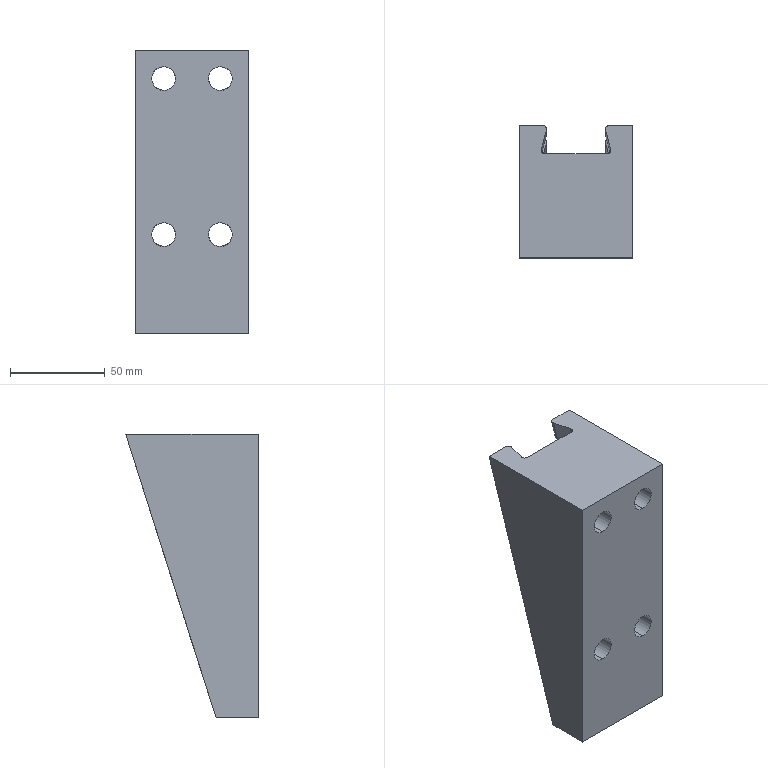Part | SolidWorks | features BaseBody 1 | 1 solid | 40 faces | box 60 x 70 x 150 mm | volume 318447 mm3 | spline 18 | plane 14 | cylinder 8 | commonest cylinder face diameters 12.5 x8